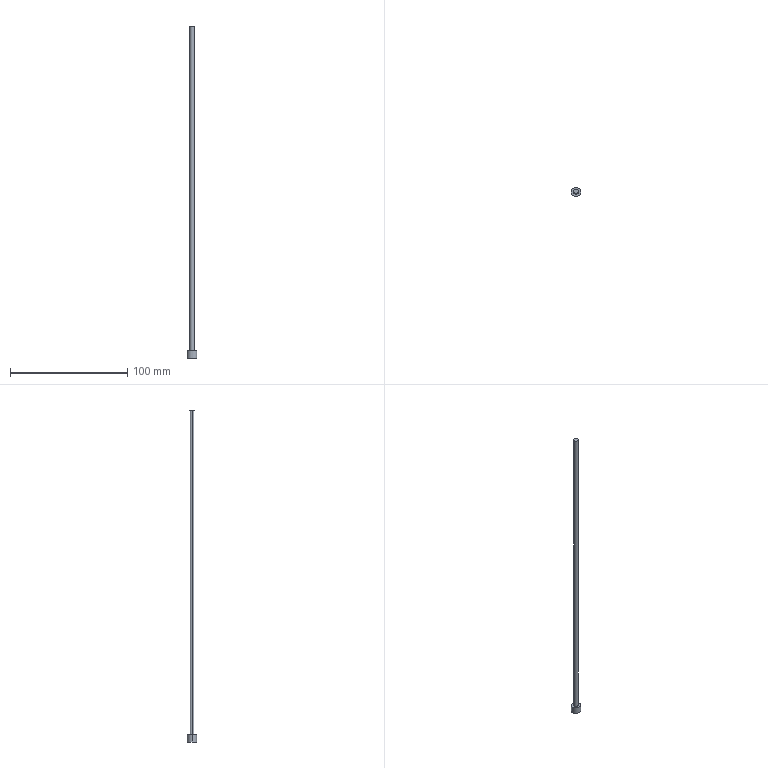Part | Creo | 1 solid | 7 faces | box 8 x 8 x 283.312 mm | volume 3786 mm3 | cylinder 4 | plane 3 | commonest cylinder face diameters 4 x2 8 x2
STEP:
#1=CARTESIAN_POINT('',(37.,-143.5,-290.));
#2=VERTEX_POINT('',#1);
#3=CARTESIAN_POINT('',(33.,-143.5,-290.));
#4=VERTEX_POINT('',#3);
#5=CARTESIAN_POINT('',(35.,-143.5,-290.));
#6=DIRECTION('',(0.,0.,-1.));
#7=DIRECTION('',(1.,0.,0.));
#8=AXIS2_PLACEMENT_3D('',#5,#6,#7);
#9=CIRCLE('',#8,2.);
#10=EDGE_CURVE('',#2,#4,#9,.T.);
#11=ORIENTED_EDGE('',*,*,#10,.T.);
#12=CARTESIAN_POINT('',(33.,-143.5,-12.688));
#13=VERTEX_POINT('',#12);
#14=CARTESIAN_POINT('',(33.,-143.5,-12.688));
#15=DIRECTION('',(0.,0.,-1.));
#16=VECTOR('',#15,277.312);
#17=LINE('',#14,#16);
#18=EDGE_CURVE('',#13,#4,#17,.T.);
#19=ORIENTED_EDGE('',*,*,#18,.F.);
#20=CARTESIAN_POINT('',(37.,-143.5,-12.688));
#21=VERTEX_POINT('',#20);
#22=CARTESIAN_POINT('',(35.,-143.5,-12.688));
#23=DIRECTION('',(0.,0.,1.));
#24=DIRECTION('',(-1.,0.,0.));
#25=AXIS2_PLACEMENT_3D('',#22,#23,#24);
#26=CIRCLE('',#25,2.);
#27=EDGE_CURVE('',#13,#21,#26,.T.);
#28=ORIENTED_EDGE('',*,*,#27,.T.);
#29=CARTESIAN_POINT('',(37.,-143.5,-12.688));
#30=DIRECTION('',(0.,0.,-1.));
#31=VECTOR('',#30,277.312);
#32=LINE('',#29,#31);
#33=EDGE_CURVE('',#21,#2,#32,.T.);
#34=ORIENTED_EDGE('',*,*,#33,.T.);
#35=EDGE_LOOP('',(#11,#19,#28,#34));
#36=FACE_OUTER_BOUND('',#35,.F.);
#37=CARTESIAN_POINT('',(35.,-143.5,-5.));
#38=DIRECTION('',(0.,0.,-1.));
#39=DIRECTION('',(1.,0.,0.));
#40=AXIS2_PLACEMENT_3D('',#37,#38,#39);
#41=CYLINDRICAL_SURFACE('',#40,2.);
#42=ADVANCED_FACE('',(#36),#41,.T.);
#43=CARTESIAN_POINT('',(39.,-143.5,-290.));
#44=VERTEX_POINT('',#43);
#45=CARTESIAN_POINT('',(31.,-143.5,-290.));
#46=VERTEX_POINT('',#45);
#47=CARTESIAN_POINT('',(35.,-143.5,-290.));
#48=DIRECTION('',(0.,0.,1.));
#49=DIRECTION('',(1.,0.,0.));
#50=AXIS2_PLACEMENT_3D('',#47,#48,#49);
#51=CIRCLE('',#50,4.);
#52=EDGE_CURVE('',#44,#46,#51,.T.);
#53=ORIENTED_EDGE('',*,*,#52,.F.);
#54=CARTESIAN_POINT('',(35.,-143.5,-290.));
#55=DIRECTION('',(0.,0.,1.));
#56=DIRECTION('',(-1.,0.,0.));
#57=AXIS2_PLACEMENT_3D('',#54,#55,#56);
#58=CIRCLE('',#57,4.);
#59=EDGE_CURVE('',#46,#44,#58,.T.);
#60=ORIENTED_EDGE('',*,*,#59,.F.);
#61=EDGE_LOOP('',(#53,#60));
#62=FACE_OUTER_BOUND('',#61,.F.);
#63=ORIENTED_EDGE('',*,*,#10,.F.);
#64=CARTESIAN_POINT('',(35.,-143.5,-290.));
#65=DIRECTION('',(0.,0.,-1.));
#66=DIRECTION('',(-1.,0.,0.));
#67=AXIS2_PLACEMENT_3D('',#64,#65,#66);
#68=CIRCLE('',#67,2.);
#69=EDGE_CURVE('',#4,#2,#68,.T.);
#70=ORIENTED_EDGE('',*,*,#69,.F.);
#71=EDGE_LOOP('',(#63,#70));
#72=FACE_BOUND('',#71,.F.);
#73=CARTESIAN_POINT('',(35.,-143.5,-290.));
#74=DIRECTION('',(0.,0.,1.));
#75=DIRECTION('',(-1.,0.,0.));
#76=AXIS2_PLACEMENT_3D('',#73,#74,#75);
#77=PLANE('',#76);
#78=ADVANCED_FACE('',(#62,#72),#77,.T.);
#79=ORIENTED_EDGE('',*,*,#69,.T.);
#80=ORIENTED_EDGE('',*,*,#33,.F.);
#81=CARTESIAN_POINT('',(35.,-143.5,-12.688));
#82=DIRECTION('',(0.,0.,1.));
#83=DIRECTION('',(1.,0.,0.));
#84=AXIS2_PLACEMENT_3D('',#81,#82,#83);
#85=CIRCLE('',#84,2.);
#86=EDGE_CURVE('',#21,#13,#85,.T.);
#87=ORIENTED_EDGE('',*,*,#86,.T.);
#88=ORIENTED_EDGE('',*,*,#18,.T.);
#89=EDGE_LOOP('',(#79,#80,#87,#88));
#90=FACE_OUTER_BOUND('',#89,.F.);
#91=CARTESIAN_POINT('',(35.,-143.5,-5.));
#92=DIRECTION('',(0.,0.,-1.));
#93=DIRECTION('',(1.,0.,0.));
#94=AXIS2_PLACEMENT_3D('',#91,#92,#93);
#95=CYLINDRICAL_SURFACE('',#94,2.);
#96=ADVANCED_FACE('',(#90),#95,.T.);
#97=ORIENTED_EDGE('',*,*,#86,.F.);
#98=ORIENTED_EDGE('',*,*,#27,.F.);
#99=EDGE_LOOP('',(#97,#98));
#100=FACE_OUTER_BOUND('',#99,.F.);
#101=CARTESIAN_POINT('',(0.,0.,-12.688));
#102=DIRECTION('',(0.,0.,1.));
#103=DIRECTION('',(0.,-1.,0.));
#104=AXIS2_PLACEMENT_3D('',#101,#102,#103);
#105=PLANE('',#104);
#106=ADVANCED_FACE('',(#100),#105,.T.);
#107=ORIENTED_EDGE('',*,*,#52,.T.);
#108=CARTESIAN_POINT('',(31.,-143.5,-296.));
#109=VERTEX_POINT('',#108);
#110=CARTESIAN_POINT('',(31.,-143.5,-296.));
#111=DIRECTION('',(0.,0.,1.));
#112=VECTOR('',#111,6.);
#113=LINE('',#110,#112);
#114=EDGE_CURVE('',#109,#46,#113,.T.);
#115=ORIENTED_EDGE('',*,*,#114,.F.);
#116=CARTESIAN_POINT('',(39.,-143.5,-296.));
#117=VERTEX_POINT('',#116);
#118=CARTESIAN_POINT('',(35.,-143.5,-296.));
#119=DIRECTION('',(0.,0.,-1.));
#120=DIRECTION('',(-1.,0.,0.));
#121=AXIS2_PLACEMENT_3D('',#118,#119,#120);
#122=CIRCLE('',#121,4.);
#123=EDGE_CURVE('',#109,#117,#122,.T.);
#124=ORIENTED_EDGE('',*,*,#123,.T.);
#125=CARTESIAN_POINT('',(39.,-143.5,-296.));
#126=DIRECTION('',(0.,0.,1.));
#127=VECTOR('',#126,6.);
#128=LINE('',#125,#127);
#129=EDGE_CURVE('',#117,#44,#128,.T.);
#130=ORIENTED_EDGE('',*,*,#129,.T.);
#131=EDGE_LOOP('',(#107,#115,#124,#130));
#132=FACE_OUTER_BOUND('',#131,.F.);
#133=CARTESIAN_POINT('',(35.,-143.5,-296.));
#134=DIRECTION('',(0.,0.,1.));
#135=DIRECTION('',(-1.,0.,0.));
#136=AXIS2_PLACEMENT_3D('',#133,#134,#135);
#137=CYLINDRICAL_SURFACE('',#136,4.);
#138=ADVANCED_FACE('',(#132),#137,.T.);
#139=ORIENTED_EDGE('',*,*,#59,.T.);
#140=ORIENTED_EDGE('',*,*,#129,.F.);
#141=CARTESIAN_POINT('',(35.,-143.5,-296.));
#142=DIRECTION('',(0.,0.,-1.));
#143=DIRECTION('',(1.,0.,0.));
#144=AXIS2_PLACEMENT_3D('',#141,#142,#143);
#145=CIRCLE('',#144,4.);
#146=EDGE_CURVE('',#117,#109,#145,.T.);
#147=ORIENTED_EDGE('',*,*,#146,.T.);
#148=ORIENTED_EDGE('',*,*,#114,.T.);
#149=EDGE_LOOP('',(#139,#140,#147,#148));
#150=FACE_OUTER_BOUND('',#149,.F.);
#151=CARTESIAN_POINT('',(35.,-143.5,-296.));
#152=DIRECTION('',(0.,0.,1.));
#153=DIRECTION('',(-1.,0.,0.));
#154=AXIS2_PLACEMENT_3D('',#151,#152,#153);
#155=CYLINDRICAL_SURFACE('',#154,4.);
#156=ADVANCED_FACE('',(#150),#155,.T.);
#157=ORIENTED_EDGE('',*,*,#146,.F.);
#158=ORIENTED_EDGE('',*,*,#123,.F.);
#159=EDGE_LOOP('',(#157,#158));
#160=FACE_OUTER_BOUND('',#159,.F.);
#161=CARTESIAN_POINT('',(7.7,-2.155,-296.));
#162=DIRECTION('',(0.,0.,1.));
#163=DIRECTION('',(0.,1.,0.));
#164=AXIS2_PLACEMENT_3D('',#161,#162,#163);
#165=PLANE('',#164);
#166=ADVANCED_FACE('',(#160),#165,.F.);
#167=CLOSED_SHELL('',(#42,#78,#96,#106,#138,#156,#166));
#168=MANIFOLD_SOLID_BREP('',#167);
#169=(LENGTH_UNIT()NAMED_UNIT(*)SI_UNIT(.MILLI.,.METRE.));
#170=UNCERTAINTY_MEASURE_WITH_UNIT(LENGTH_MEASURE(0.02835),#169,'','');
#171=(NAMED_UNIT(*)PLANE_ANGLE_UNIT()SI_UNIT($,.RADIAN.));
#172=PLANE_ANGLE_MEASURE_WITH_UNIT(PLANE_ANGLE_MEASURE(0.01745),#171);
#173=(CONVERSION_BASED_UNIT('DEGREE',#172)NAMED_UNIT(*)PLANE_ANGLE_UNIT());
#174=(NAMED_UNIT(*)SI_UNIT($,.STERADIAN.)SOLID_ANGLE_UNIT());
#175=(GEOMETRIC_REPRESENTATION_CONTEXT(3)GLOBAL_UNCERTAINTY_ASSIGNED_CONTEXT((#170))GLOBAL_UNIT_ASSIGNED_CONTEXT((#169,#173,#174))REPRESENTATION_CONTEXT('',''));
#176=ADVANCED_BREP_SHAPE_REPRESENTATION('',(#168),#175);